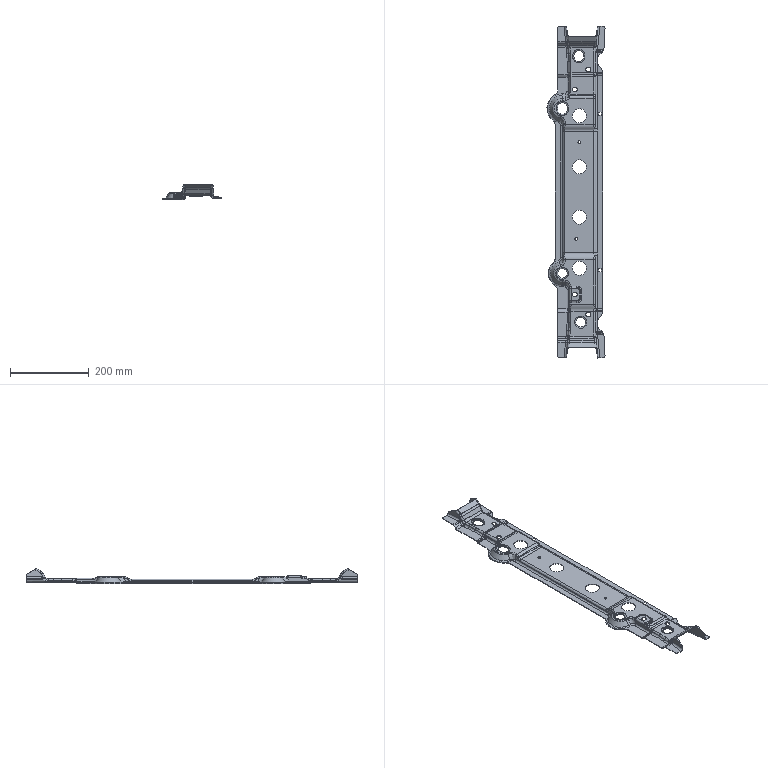Part | 1 solid | 712 faces | box 147.882 x 845.314 x 38.578 mm | volume 158087 mm3 | spline 314 | cylinder 256 | plane 114 | sphere 24 | torus 4 | commonest cylinder face diameters 10 x84 7 x48 13 x36 20 x14 12 x10 30 x9